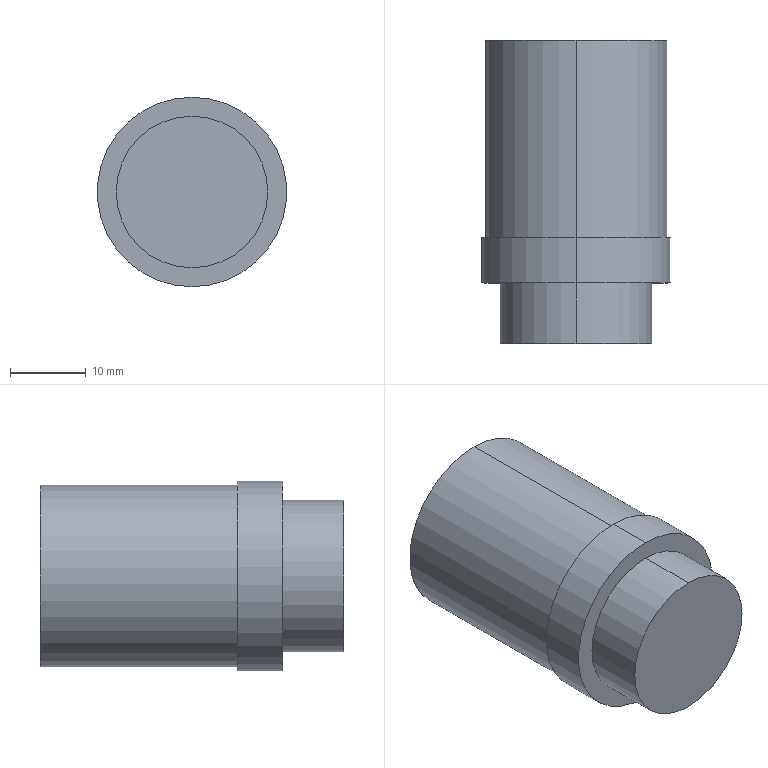Part | SolidWorks | features Revolution 1 | 1 solid | 10 faces | box 25 x 40 x 25 mm | volume 17221 mm3 | cylinder 6 | plane 4 | commonest cylinder face diameters 20 x2 24 x2 25 x2
STEP:
#1=CARTESIAN_POINT('',(0.,8.,-10.));
#2=VERTEX_POINT('',#1);
#3=CARTESIAN_POINT('',(0.,8.,10.));
#4=VERTEX_POINT('',#3);
#5=CARTESIAN_POINT('',(0.,8.,0.));
#6=DIRECTION('',(0.,-1.,0.));
#7=DIRECTION('',(0.,0.,-1.));
#8=AXIS2_PLACEMENT_3D('',#5,#6,#7);
#9=CIRCLE('',#8,10.);
#10=EDGE_CURVE('',#2,#4,#9,.T.);
#11=ORIENTED_EDGE('',*,*,#10,.T.);
#12=CARTESIAN_POINT('',(0.,0.,10.));
#13=VERTEX_POINT('',#12);
#14=CARTESIAN_POINT('',(0.,0.,10.));
#15=DIRECTION('',(0.,-1.,0.));
#16=VECTOR('',#15,1000.);
#17=LINE('',#14,#16);
#18=EDGE_CURVE('',#4,#13,#17,.T.);
#19=ORIENTED_EDGE('',*,*,#18,.T.);
#20=CARTESIAN_POINT('',(0.,0.,-10.));
#21=VERTEX_POINT('',#20);
#22=CARTESIAN_POINT('',(0.,0.,0.));
#23=DIRECTION('',(0.,-1.,0.));
#24=DIRECTION('',(0.,0.,-1.));
#25=AXIS2_PLACEMENT_3D('',#22,#23,#24);
#26=CIRCLE('',#25,10.);
#27=EDGE_CURVE('',#21,#13,#26,.T.);
#28=ORIENTED_EDGE('',*,*,#27,.F.);
#29=CARTESIAN_POINT('',(0.,0.,-10.));
#30=DIRECTION('',(0.,-1.,0.));
#31=VECTOR('',#30,1000.);
#32=LINE('',#29,#31);
#33=EDGE_CURVE('',#2,#21,#32,.T.);
#34=ORIENTED_EDGE('',*,*,#33,.F.);
#35=EDGE_LOOP('',(#11,#19,#28,#34));
#36=FACE_OUTER_BOUND('',#35,.T.);
#37=CARTESIAN_POINT('',(0.,0.,0.));
#38=DIRECTION('',(0.,-1.,0.));
#39=DIRECTION('',(0.,0.,-1.));
#40=AXIS2_PLACEMENT_3D('',#37,#38,#39);
#41=CYLINDRICAL_SURFACE('',#40,10.);
#42=ADVANCED_FACE('',(#36),#41,.T.);
#43=CARTESIAN_POINT('',(0.,14.,-12.5));
#44=VERTEX_POINT('',#43);
#45=CARTESIAN_POINT('',(0.,14.,12.5));
#46=VERTEX_POINT('',#45);
#47=CARTESIAN_POINT('',(0.,14.,0.));
#48=DIRECTION('',(0.,-1.,0.));
#49=DIRECTION('',(0.,0.,-1.));
#50=AXIS2_PLACEMENT_3D('',#47,#48,#49);
#51=CIRCLE('',#50,12.5);
#52=EDGE_CURVE('',#44,#46,#51,.T.);
#53=ORIENTED_EDGE('',*,*,#52,.T.);
#54=CARTESIAN_POINT('',(0.,8.,12.5));
#55=VERTEX_POINT('',#54);
#56=CARTESIAN_POINT('',(0.,0.,12.5));
#57=DIRECTION('',(0.,-1.,0.));
#58=VECTOR('',#57,1000.);
#59=LINE('',#56,#58);
#60=EDGE_CURVE('',#46,#55,#59,.T.);
#61=ORIENTED_EDGE('',*,*,#60,.T.);
#62=CARTESIAN_POINT('',(0.,8.,-12.5));
#63=VERTEX_POINT('',#62);
#64=CARTESIAN_POINT('',(0.,8.,0.));
#65=DIRECTION('',(0.,-1.,0.));
#66=DIRECTION('',(0.,0.,-1.));
#67=AXIS2_PLACEMENT_3D('',#64,#65,#66);
#68=CIRCLE('',#67,12.5);
#69=EDGE_CURVE('',#63,#55,#68,.T.);
#70=ORIENTED_EDGE('',*,*,#69,.F.);
#71=CARTESIAN_POINT('',(0.,0.,-12.5));
#72=DIRECTION('',(0.,-1.,0.));
#73=VECTOR('',#72,1000.);
#74=LINE('',#71,#73);
#75=EDGE_CURVE('',#44,#63,#74,.T.);
#76=ORIENTED_EDGE('',*,*,#75,.F.);
#77=EDGE_LOOP('',(#53,#61,#70,#76));
#78=FACE_OUTER_BOUND('',#77,.T.);
#79=CARTESIAN_POINT('',(0.,0.,0.));
#80=DIRECTION('',(0.,-1.,0.));
#81=DIRECTION('',(0.,0.,-1.));
#82=AXIS2_PLACEMENT_3D('',#79,#80,#81);
#83=CYLINDRICAL_SURFACE('',#82,12.5);
#84=ADVANCED_FACE('',(#78),#83,.T.);
#85=CARTESIAN_POINT('',(0.,40.,-12.));
#86=VERTEX_POINT('',#85);
#87=CARTESIAN_POINT('',(0.,40.,12.));
#88=VERTEX_POINT('',#87);
#89=CARTESIAN_POINT('',(0.,40.,0.));
#90=DIRECTION('',(0.,-1.,0.));
#91=DIRECTION('',(0.,0.,-1.));
#92=AXIS2_PLACEMENT_3D('',#89,#90,#91);
#93=CIRCLE('',#92,12.);
#94=EDGE_CURVE('',#86,#88,#93,.T.);
#95=ORIENTED_EDGE('',*,*,#94,.T.);
#96=CARTESIAN_POINT('',(0.,14.,12.));
#97=VERTEX_POINT('',#96);
#98=CARTESIAN_POINT('',(0.,0.,12.));
#99=DIRECTION('',(0.,-1.,0.));
#100=VECTOR('',#99,1000.);
#101=LINE('',#98,#100);
#102=EDGE_CURVE('',#88,#97,#101,.T.);
#103=ORIENTED_EDGE('',*,*,#102,.T.);
#104=CARTESIAN_POINT('',(0.,14.,-12.));
#105=VERTEX_POINT('',#104);
#106=CARTESIAN_POINT('',(0.,14.,0.));
#107=DIRECTION('',(0.,-1.,0.));
#108=DIRECTION('',(0.,0.,-1.));
#109=AXIS2_PLACEMENT_3D('',#106,#107,#108);
#110=CIRCLE('',#109,12.);
#111=EDGE_CURVE('',#105,#97,#110,.T.);
#112=ORIENTED_EDGE('',*,*,#111,.F.);
#113=CARTESIAN_POINT('',(0.,0.,-12.));
#114=DIRECTION('',(0.,-1.,0.));
#115=VECTOR('',#114,1000.);
#116=LINE('',#113,#115);
#117=EDGE_CURVE('',#86,#105,#116,.T.);
#118=ORIENTED_EDGE('',*,*,#117,.F.);
#119=EDGE_LOOP('',(#95,#103,#112,#118));
#120=FACE_OUTER_BOUND('',#119,.T.);
#121=CARTESIAN_POINT('',(0.,0.,0.));
#122=DIRECTION('',(0.,-1.,0.));
#123=DIRECTION('',(0.,0.,-1.));
#124=AXIS2_PLACEMENT_3D('',#121,#122,#123);
#125=CYLINDRICAL_SURFACE('',#124,12.);
#126=ADVANCED_FACE('',(#120),#125,.T.);
#127=ORIENTED_EDGE('',*,*,#94,.F.);
#128=CARTESIAN_POINT('',(0.,40.,0.));
#129=DIRECTION('',(0.,-1.,0.));
#130=DIRECTION('',(0.,0.,-1.));
#131=AXIS2_PLACEMENT_3D('',#128,#129,#130);
#132=CIRCLE('',#131,12.);
#133=EDGE_CURVE('',#88,#86,#132,.T.);
#134=ORIENTED_EDGE('',*,*,#133,.F.);
#135=EDGE_LOOP('',(#127,#134));
#136=FACE_OUTER_BOUND('',#135,.T.);
#137=CARTESIAN_POINT('',(0.,40.,0.));
#138=DIRECTION('',(0.,-1.,0.));
#139=DIRECTION('',(0.,0.,-1.));
#140=AXIS2_PLACEMENT_3D('',#137,#138,#139);
#141=PLANE('',#140);
#142=ADVANCED_FACE('',(#136),#141,.F.);
#143=ORIENTED_EDGE('',*,*,#102,.F.);
#144=ORIENTED_EDGE('',*,*,#133,.T.);
#145=ORIENTED_EDGE('',*,*,#117,.T.);
#146=CARTESIAN_POINT('',(0.,14.,0.));
#147=DIRECTION('',(0.,-1.,0.));
#148=DIRECTION('',(0.,0.,-1.));
#149=AXIS2_PLACEMENT_3D('',#146,#147,#148);
#150=CIRCLE('',#149,12.);
#151=EDGE_CURVE('',#97,#105,#150,.T.);
#152=ORIENTED_EDGE('',*,*,#151,.F.);
#153=EDGE_LOOP('',(#143,#144,#145,#152));
#154=FACE_OUTER_BOUND('',#153,.T.);
#155=CARTESIAN_POINT('',(0.,0.,0.));
#156=DIRECTION('',(0.,-1.,0.));
#157=DIRECTION('',(0.,0.,-1.));
#158=AXIS2_PLACEMENT_3D('',#155,#156,#157);
#159=CYLINDRICAL_SURFACE('',#158,12.);
#160=ADVANCED_FACE('',(#154),#159,.T.);
#161=ORIENTED_EDGE('',*,*,#52,.F.);
#162=CARTESIAN_POINT('',(0.,14.,0.));
#163=DIRECTION('',(0.,-1.,0.));
#164=DIRECTION('',(0.,0.,-1.));
#165=AXIS2_PLACEMENT_3D('',#162,#163,#164);
#166=CIRCLE('',#165,12.5);
#167=EDGE_CURVE('',#46,#44,#166,.T.);
#168=ORIENTED_EDGE('',*,*,#167,.F.);
#169=EDGE_LOOP('',(#161,#168));
#170=FACE_OUTER_BOUND('',#169,.T.);
#171=ORIENTED_EDGE('',*,*,#111,.T.);
#172=ORIENTED_EDGE('',*,*,#151,.T.);
#173=EDGE_LOOP('',(#171,#172));
#174=FACE_BOUND('',#173,.T.);
#175=CARTESIAN_POINT('',(-12.,14.,0.));
#176=DIRECTION('',(0.,-1.,0.));
#177=DIRECTION('',(0.,0.,-1.));
#178=AXIS2_PLACEMENT_3D('',#175,#176,#177);
#179=PLANE('',#178);
#180=ADVANCED_FACE('',(#170,#174),#179,.F.);
#181=ORIENTED_EDGE('',*,*,#60,.F.);
#182=ORIENTED_EDGE('',*,*,#167,.T.);
#183=ORIENTED_EDGE('',*,*,#75,.T.);
#184=CARTESIAN_POINT('',(0.,8.,0.));
#185=DIRECTION('',(0.,-1.,0.));
#186=DIRECTION('',(0.,0.,-1.));
#187=AXIS2_PLACEMENT_3D('',#184,#185,#186);
#188=CIRCLE('',#187,12.5);
#189=EDGE_CURVE('',#55,#63,#188,.T.);
#190=ORIENTED_EDGE('',*,*,#189,.F.);
#191=EDGE_LOOP('',(#181,#182,#183,#190));
#192=FACE_OUTER_BOUND('',#191,.T.);
#193=CARTESIAN_POINT('',(0.,0.,0.));
#194=DIRECTION('',(0.,-1.,0.));
#195=DIRECTION('',(0.,0.,-1.));
#196=AXIS2_PLACEMENT_3D('',#193,#194,#195);
#197=CYLINDRICAL_SURFACE('',#196,12.5);
#198=ADVANCED_FACE('',(#192),#197,.T.);
#199=ORIENTED_EDGE('',*,*,#10,.F.);
#200=CARTESIAN_POINT('',(0.,8.,0.));
#201=DIRECTION('',(0.,-1.,0.));
#202=DIRECTION('',(0.,0.,-1.));
#203=AXIS2_PLACEMENT_3D('',#200,#201,#202);
#204=CIRCLE('',#203,10.);
#205=EDGE_CURVE('',#4,#2,#204,.T.);
#206=ORIENTED_EDGE('',*,*,#205,.F.);
#207=EDGE_LOOP('',(#199,#206));
#208=FACE_BOUND('',#207,.T.);
#209=ORIENTED_EDGE('',*,*,#69,.T.);
#210=ORIENTED_EDGE('',*,*,#189,.T.);
#211=EDGE_LOOP('',(#209,#210));
#212=FACE_OUTER_BOUND('',#211,.T.);
#213=CARTESIAN_POINT('',(-12.5,8.,0.));
#214=DIRECTION('',(0.,1.,0.));
#215=DIRECTION('',(0.,0.,1.));
#216=AXIS2_PLACEMENT_3D('',#213,#214,#215);
#217=PLANE('',#216);
#218=ADVANCED_FACE('',(#208,#212),#217,.F.);
#219=ORIENTED_EDGE('',*,*,#18,.F.);
#220=ORIENTED_EDGE('',*,*,#205,.T.);
#221=ORIENTED_EDGE('',*,*,#33,.T.);
#222=CARTESIAN_POINT('',(0.,0.,0.));
#223=DIRECTION('',(0.,-1.,0.));
#224=DIRECTION('',(0.,0.,-1.));
#225=AXIS2_PLACEMENT_3D('',#222,#223,#224);
#226=CIRCLE('',#225,10.);
#227=EDGE_CURVE('',#13,#21,#226,.T.);
#228=ORIENTED_EDGE('',*,*,#227,.F.);
#229=EDGE_LOOP('',(#219,#220,#221,#228));
#230=FACE_OUTER_BOUND('',#229,.T.);
#231=CARTESIAN_POINT('',(0.,0.,0.));
#232=DIRECTION('',(0.,-1.,0.));
#233=DIRECTION('',(0.,0.,-1.));
#234=AXIS2_PLACEMENT_3D('',#231,#232,#233);
#235=CYLINDRICAL_SURFACE('',#234,10.);
#236=ADVANCED_FACE('',(#230),#235,.T.);
#237=ORIENTED_EDGE('',*,*,#27,.T.);
#238=ORIENTED_EDGE('',*,*,#227,.T.);
#239=EDGE_LOOP('',(#237,#238));
#240=FACE_OUTER_BOUND('',#239,.T.);
#241=CARTESIAN_POINT('',(-10.,0.,0.));
#242=DIRECTION('',(0.,1.,0.));
#243=DIRECTION('',(0.,0.,1.));
#244=AXIS2_PLACEMENT_3D('',#241,#242,#243);
#245=PLANE('',#244);
#246=ADVANCED_FACE('',(#240),#245,.F.);
#247=CLOSED_SHELL('',(#42,#84,#126,#142,#160,#180,#198,#218,#236,#246));
#248=MANIFOLD_SOLID_BREP('',#247);
#249=CARTESIAN_POINT('',(0.,0.,0.));
#250=DIRECTION('',(0.,0.,1.));
#251=DIRECTION('',(1.,0.,0.));
#252=AXIS2_PLACEMENT_3D('',#249,#250,#251);
#253=(LENGTH_UNIT()NAMED_UNIT(*)SI_UNIT(.MILLI.,.METRE.));
#254=UNCERTAINTY_MEASURE_WITH_UNIT(LENGTH_MEASURE(0.00001),#253,'','');
#255=(NAMED_UNIT(*)PLANE_ANGLE_UNIT()SI_UNIT($,.RADIAN.));
#256=(NAMED_UNIT(*)SI_UNIT($,.STERADIAN.)SOLID_ANGLE_UNIT());
#257=(GEOMETRIC_REPRESENTATION_CONTEXT(3)GLOBAL_UNCERTAINTY_ASSIGNED_CONTEXT((#254))GLOBAL_UNIT_ASSIGNED_CONTEXT((#253,#255,#256))REPRESENTATION_CONTEXT('',''));
#258=ADVANCED_BREP_SHAPE_REPRESENTATION('',(#248,#252),#257);